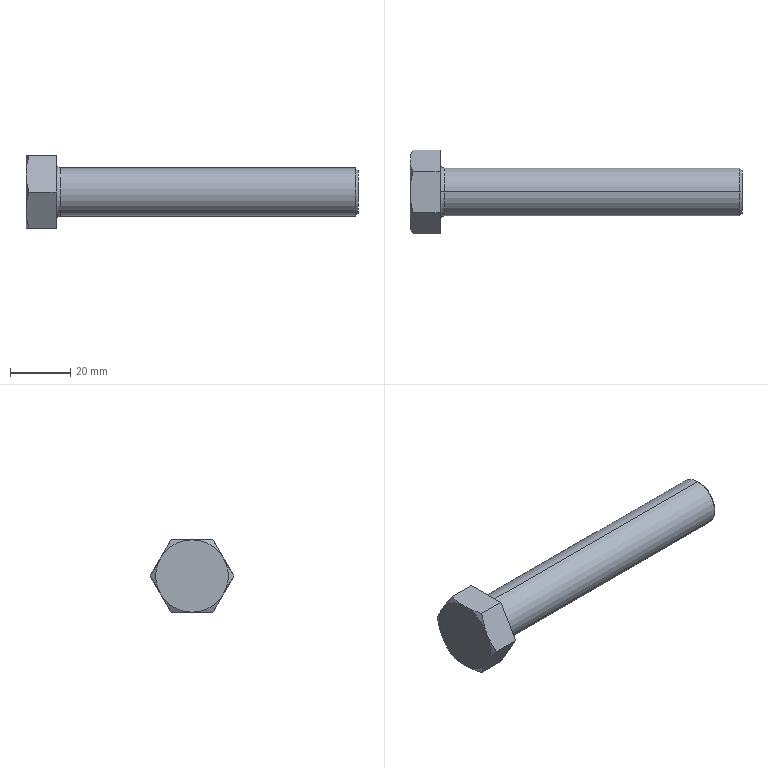Part | SolidWorks | features Chamfer 2, RevCut 2, Revolution 2, Extrusion 1, ICE 1 | 1 solid | 21 faces | box 110 x 27.713 x 24 mm | volume 25081 mm3 | plane 9 | cone 8 | cylinder 2 | torus 2 | commonest cylinder face diameters 16 x2
STEP:
#1=CARTESIAN_POINT('',(110.,0.,-7.111));
#2=VERTEX_POINT('',#1);
#3=CARTESIAN_POINT('',(110.,0.,7.111));
#4=VERTEX_POINT('',#3);
#5=CARTESIAN_POINT('',(110.,0.,0.));
#6=DIRECTION('',(1.,0.,0.));
#7=DIRECTION('',(0.,0.,1.));
#8=AXIS2_PLACEMENT_3D('',#5,#6,#7);
#9=CIRCLE('',#8,7.111);
#10=EDGE_CURVE('',#2,#4,#9,.T.);
#11=ORIENTED_EDGE('',*,*,#10,.F.);
#12=CARTESIAN_POINT('',(109.111,0.,-8.));
#13=VERTEX_POINT('',#12);
#14=CARTESIAN_POINT('',(109.111,0.,-8.));
#15=DIRECTION('',(-0.7071,0.,-0.7071));
#16=VECTOR('',#15,1000.);
#17=LINE('',#14,#16);
#18=EDGE_CURVE('',#2,#13,#17,.T.);
#19=ORIENTED_EDGE('',*,*,#18,.T.);
#20=CARTESIAN_POINT('',(109.111,0.,8.));
#21=VERTEX_POINT('',#20);
#22=CARTESIAN_POINT('',(109.111,0.,0.));
#23=DIRECTION('',(-1.,0.,0.));
#24=DIRECTION('',(0.,0.,1.));
#25=AXIS2_PLACEMENT_3D('',#22,#23,#24);
#26=CIRCLE('',#25,8.);
#27=EDGE_CURVE('',#21,#13,#26,.T.);
#28=ORIENTED_EDGE('',*,*,#27,.F.);
#29=CARTESIAN_POINT('',(109.111,0.,8.));
#30=DIRECTION('',(-0.7071,0.,0.7071));
#31=VECTOR('',#30,1000.);
#32=LINE('',#29,#31);
#33=EDGE_CURVE('',#4,#21,#32,.T.);
#34=ORIENTED_EDGE('',*,*,#33,.F.);
#35=EDGE_LOOP('',(#11,#19,#28,#34));
#36=FACE_OUTER_BOUND('',#35,.T.);
#37=CARTESIAN_POINT('',(109.111,0.,0.));
#38=DIRECTION('',(-1.,0.,0.));
#39=DIRECTION('',(0.,0.,1.));
#40=AXIS2_PLACEMENT_3D('',#37,#38,#39);
#41=CONICAL_SURFACE('',#40,8.,0.7854);
#42=ADVANCED_FACE('',(#36),#41,.T.);
#43=ORIENTED_EDGE('',*,*,#27,.T.);
#44=CARTESIAN_POINT('',(11.35,0.,-8.));
#45=VERTEX_POINT('',#44);
#46=CARTESIAN_POINT('',(10.,0.,-8.));
#47=DIRECTION('',(-1.,0.,0.));
#48=VECTOR('',#47,1000.);
#49=LINE('',#46,#48);
#50=EDGE_CURVE('',#13,#45,#49,.T.);
#51=ORIENTED_EDGE('',*,*,#50,.T.);
#52=CARTESIAN_POINT('',(11.35,0.,8.));
#53=VERTEX_POINT('',#52);
#54=CARTESIAN_POINT('',(11.35,0.,0.));
#55=DIRECTION('',(-1.,0.,0.));
#56=DIRECTION('',(0.,0.,1.));
#57=AXIS2_PLACEMENT_3D('',#54,#55,#56);
#58=CIRCLE('',#57,8.);
#59=EDGE_CURVE('',#53,#45,#58,.T.);
#60=ORIENTED_EDGE('',*,*,#59,.F.);
#61=CARTESIAN_POINT('',(10.,0.,8.));
#62=DIRECTION('',(-1.,0.,0.));
#63=VECTOR('',#62,1000.);
#64=LINE('',#61,#63);
#65=EDGE_CURVE('',#21,#53,#64,.T.);
#66=ORIENTED_EDGE('',*,*,#65,.F.);
#67=EDGE_LOOP('',(#43,#51,#60,#66));
#68=FACE_OUTER_BOUND('',#67,.T.);
#69=CARTESIAN_POINT('',(10.,0.,0.));
#70=DIRECTION('',(-1.,0.,0.));
#71=DIRECTION('',(0.,0.,1.));
#72=AXIS2_PLACEMENT_3D('',#69,#70,#71);
#73=CYLINDRICAL_SURFACE('',#72,8.);
#74=ADVANCED_FACE('',(#68),#73,.T.);
#75=CARTESIAN_POINT('',(10.,0.,-9.35));
#76=VERTEX_POINT('',#75);
#77=CARTESIAN_POINT('',(10.,0.,9.35));
#78=VERTEX_POINT('',#77);
#79=CARTESIAN_POINT('',(10.,0.,0.));
#80=DIRECTION('',(-1.,0.,0.));
#81=DIRECTION('',(0.,0.,1.));
#82=AXIS2_PLACEMENT_3D('',#79,#80,#81);
#83=CIRCLE('',#82,9.35);
#84=EDGE_CURVE('',#76,#78,#83,.T.);
#85=ORIENTED_EDGE('',*,*,#84,.F.);
#86=CARTESIAN_POINT('',(11.35,0.,-9.35));
#87=DIRECTION('',(0.,1.,0.));
#88=DIRECTION('',(0.,0.,1.));
#89=AXIS2_PLACEMENT_3D('',#86,#87,#88);
#90=CIRCLE('',#89,1.35);
#91=EDGE_CURVE('',#76,#45,#90,.T.);
#92=ORIENTED_EDGE('',*,*,#91,.T.);
#93=CARTESIAN_POINT('',(11.35,0.,0.));
#94=DIRECTION('',(-1.,0.,0.));
#95=DIRECTION('',(0.,0.,1.));
#96=AXIS2_PLACEMENT_3D('',#93,#94,#95);
#97=CIRCLE('',#96,8.);
#98=EDGE_CURVE('',#45,#53,#97,.T.);
#99=ORIENTED_EDGE('',*,*,#98,.T.);
#100=CARTESIAN_POINT('',(11.35,0.,9.35));
#101=DIRECTION('',(0.,-1.,0.));
#102=DIRECTION('',(0.,0.,-1.));
#103=AXIS2_PLACEMENT_3D('',#100,#101,#102);
#104=CIRCLE('',#103,1.35);
#105=EDGE_CURVE('',#78,#53,#104,.T.);
#106=ORIENTED_EDGE('',*,*,#105,.F.);
#107=EDGE_LOOP('',(#85,#92,#99,#106));
#108=FACE_OUTER_BOUND('',#107,.T.);
#109=CARTESIAN_POINT('',(11.35,0.,0.));
#110=DIRECTION('',(-1.,0.,0.));
#111=DIRECTION('',(0.,0.,1.));
#112=AXIS2_PLACEMENT_3D('',#109,#110,#111);
#113=TOROIDAL_SURFACE('',#112,9.35,1.35);
#114=ADVANCED_FACE('',(#108),#113,.F.);
#115=CARTESIAN_POINT('',(10.,-6.928,-12.));
#116=VERTEX_POINT('',#115);
#117=CARTESIAN_POINT('',(10.,6.928,-12.));
#118=VERTEX_POINT('',#117);
#119=CARTESIAN_POINT('',(10.,-6.928,-12.));
#120=DIRECTION('',(0.,1.,0.));
#121=VECTOR('',#120,1000.);
#122=LINE('',#119,#121);
#123=EDGE_CURVE('',#116,#118,#122,.T.);
#124=ORIENTED_EDGE('',*,*,#123,.T.);
#125=CARTESIAN_POINT('',(10.,13.856,0.));
#126=VERTEX_POINT('',#125);
#127=CARTESIAN_POINT('',(10.,6.928,-12.));
#128=DIRECTION('',(0.,0.5,0.866));
#129=VECTOR('',#128,1000.);
#130=LINE('',#127,#129);
#131=EDGE_CURVE('',#118,#126,#130,.T.);
#132=ORIENTED_EDGE('',*,*,#131,.T.);
#133=CARTESIAN_POINT('',(10.,6.928,12.));
#134=VERTEX_POINT('',#133);
#135=CARTESIAN_POINT('',(10.,13.856,0.));
#136=DIRECTION('',(0.,-0.5,0.866));
#137=VECTOR('',#136,1000.);
#138=LINE('',#135,#137);
#139=EDGE_CURVE('',#126,#134,#138,.T.);
#140=ORIENTED_EDGE('',*,*,#139,.T.);
#141=CARTESIAN_POINT('',(10.,-6.928,12.));
#142=VERTEX_POINT('',#141);
#143=CARTESIAN_POINT('',(10.,6.928,12.));
#144=DIRECTION('',(0.,-1.,0.));
#145=VECTOR('',#144,1000.);
#146=LINE('',#143,#145);
#147=EDGE_CURVE('',#134,#142,#146,.T.);
#148=ORIENTED_EDGE('',*,*,#147,.T.);
#149=CARTESIAN_POINT('',(10.,-13.856,0.));
#150=VERTEX_POINT('',#149);
#151=CARTESIAN_POINT('',(10.,-6.928,12.));
#152=DIRECTION('',(0.,-0.5,-0.866));
#153=VECTOR('',#152,1000.);
#154=LINE('',#151,#153);
#155=EDGE_CURVE('',#142,#150,#154,.T.);
#156=ORIENTED_EDGE('',*,*,#155,.T.);
#157=CARTESIAN_POINT('',(10.,-13.856,0.));
#158=DIRECTION('',(0.,0.5,-0.866));
#159=VECTOR('',#158,1000.);
#160=LINE('',#157,#159);
#161=EDGE_CURVE('',#150,#116,#160,.T.);
#162=ORIENTED_EDGE('',*,*,#161,.T.);
#163=EDGE_LOOP('',(#124,#132,#140,#148,#156,#162));
#164=FACE_OUTER_BOUND('',#163,.T.);
#165=CARTESIAN_POINT('',(10.,0.,0.));
#166=DIRECTION('',(-1.,0.,0.));
#167=DIRECTION('',(0.,0.,1.));
#168=AXIS2_PLACEMENT_3D('',#165,#166,#167);
#169=CIRCLE('',#168,9.35);
#170=EDGE_CURVE('',#78,#76,#169,.T.);
#171=ORIENTED_EDGE('',*,*,#170,.T.);
#172=ORIENTED_EDGE('',*,*,#84,.T.);
#173=EDGE_LOOP('',(#171,#172));
#174=FACE_BOUND('',#173,.T.);
#175=CARTESIAN_POINT('',(10.,6.928,-12.));
#176=DIRECTION('',(1.,0.,0.));
#177=DIRECTION('',(0.,0.,-1.));
#178=AXIS2_PLACEMENT_3D('',#175,#176,#177);
#179=PLANE('',#178);
#180=ADVANCED_FACE('',(#164,#174),#179,.T.);
#181=CARTESIAN_POINT('',(1.072,6.928,-12.));
#182=VERTEX_POINT('',#181);
#183=CARTESIAN_POINT('',(0.,0.,-12.));
#184=VERTEX_POINT('',#183);
#185=CARTESIAN_POINT('',(1.072,6.928,-12.));
#186=CARTESIAN_POINT('',(0.7484,5.808,-12.));
#187=CARTESIAN_POINT('',(0.4791,4.673,-12.));
#188=CARTESIAN_POINT('',(0.1974,2.937,-12.));
#189=CARTESIAN_POINT('',(0.1238,2.353,-12.));
#190=CARTESIAN_POINT('',(0.0249,1.173,-12.));
#191=CARTESIAN_POINT('',(0.,0.5858,-12.));
#192=CARTESIAN_POINT('',(0.,0.,-12.));
#193=B_SPLINE_CURVE_WITH_KNOTS('',3,(#185,#186,#187,#188,#189,#190,#191,#192),.UNSPECIFIED.,.F.,.F.,(4,2,2,4),(0.005049,0.008547,0.0103,0.01204),.UNSPECIFIED.);
#194=EDGE_CURVE('',#182,#184,#193,.T.);
#195=ORIENTED_EDGE('',*,*,#194,.F.);
#196=CARTESIAN_POINT('',(10.,6.928,-12.));
#197=DIRECTION('',(-1.,0.,0.));
#198=VECTOR('',#197,1000.);
#199=LINE('',#196,#198);
#200=EDGE_CURVE('',#118,#182,#199,.T.);
#201=ORIENTED_EDGE('',*,*,#200,.F.);
#202=ORIENTED_EDGE('',*,*,#123,.F.);
#203=CARTESIAN_POINT('',(1.072,-6.928,-12.));
#204=VERTEX_POINT('',#203);
#205=CARTESIAN_POINT('',(10.,-6.928,-12.));
#206=DIRECTION('',(-1.,0.,0.));
#207=VECTOR('',#206,1000.);
#208=LINE('',#205,#207);
#209=EDGE_CURVE('',#116,#204,#208,.T.);
#210=ORIENTED_EDGE('',*,*,#209,.T.);
#211=CARTESIAN_POINT('',(0.,0.,-12.));
#212=CARTESIAN_POINT('',(0.,-1.171,-12.));
#213=CARTESIAN_POINT('',(0.1006,-2.334,-12.));
#214=CARTESIAN_POINT('',(0.4737,-4.647,-12.));
#215=CARTESIAN_POINT('',(0.7465,-5.801,-12.));
#216=CARTESIAN_POINT('',(1.072,-6.928,-12.));
#217=B_SPLINE_CURVE_WITH_KNOTS('',3,(#211,#212,#213,#214,#215,#216),.UNSPECIFIED.,.F.,.F.,(4,2,4),(0.01204,0.01554,0.01904),.UNSPECIFIED.);
#218=EDGE_CURVE('',#184,#204,#217,.T.);
#219=ORIENTED_EDGE('',*,*,#218,.F.);
#220=EDGE_LOOP('',(#195,#201,#202,#210,#219));
#221=FACE_OUTER_BOUND('',#220,.T.);
#222=CARTESIAN_POINT('',(10.,-6.928,-12.));
#223=DIRECTION('',(0.,0.,1.));
#224=DIRECTION('',(0.,-1.,0.));
#225=AXIS2_PLACEMENT_3D('',#222,#223,#224);
#226=PLANE('',#225);
#227=ADVANCED_FACE('',(#221),#226,.F.);
#228=CARTESIAN_POINT('',(1.072,13.856,0.));
#229=VERTEX_POINT('',#228);
#230=CARTESIAN_POINT('',(0.,10.392,-6.));
#231=VERTEX_POINT('',#230);
#232=CARTESIAN_POINT('',(1.072,13.856,0.));
#233=CARTESIAN_POINT('',(0.7446,13.29,-0.9815));
#234=CARTESIAN_POINT('',(0.4751,12.719,-1.97));
#235=CARTESIAN_POINT('',(0.1021,11.565,-3.968));
#236=CARTESIAN_POINT('',(0.,10.982,-4.978));
#237=CARTESIAN_POINT('',(0.,10.392,-6.));
#238=B_SPLINE_CURVE_WITH_KNOTS('',3,(#232,#233,#234,#235,#236,#237),.UNSPECIFIED.,.F.,.F.,(4,2,4),(0.000000238,0.003505,0.00701),.UNSPECIFIED.);
#239=EDGE_CURVE('',#229,#231,#238,.T.);
#240=ORIENTED_EDGE('',*,*,#239,.F.);
#241=CARTESIAN_POINT('',(10.,13.856,0.));
#242=DIRECTION('',(-1.,0.,0.));
#243=VECTOR('',#242,1000.);
#244=LINE('',#241,#243);
#245=EDGE_CURVE('',#126,#229,#244,.T.);
#246=ORIENTED_EDGE('',*,*,#245,.F.);
#247=ORIENTED_EDGE('',*,*,#131,.F.);
#248=ORIENTED_EDGE('',*,*,#200,.T.);
#249=CARTESIAN_POINT('',(0.,10.392,-6.));
#250=CARTESIAN_POINT('',(0.,10.098,-6.509));
#251=CARTESIAN_POINT('',(0.02533,9.803,-7.021));
#252=CARTESIAN_POINT('',(0.1234,9.219,-8.033));
#253=CARTESIAN_POINT('',(0.196,8.929,-8.535));
#254=CARTESIAN_POINT('',(0.476,8.063,-10.034));
#255=CARTESIAN_POINT('',(0.7454,7.493,-11.021));
#256=CARTESIAN_POINT('',(1.072,6.928,-12.));
#257=B_SPLINE_CURVE_WITH_KNOTS('',3,(#249,#250,#251,#252,#253,#254,#255,#256),.UNSPECIFIED.,.F.,.F.,(4,2,2,4),(0.00701,0.008756,0.0105,0.01399),.UNSPECIFIED.);
#258=EDGE_CURVE('',#231,#182,#257,.T.);
#259=ORIENTED_EDGE('',*,*,#258,.F.);
#260=EDGE_LOOP('',(#240,#246,#247,#248,#259));
#261=FACE_OUTER_BOUND('',#260,.T.);
#262=CARTESIAN_POINT('',(10.,6.928,-12.));
#263=DIRECTION('',(0.,-0.866,0.5));
#264=DIRECTION('',(0.,-0.5,-0.866));
#265=AXIS2_PLACEMENT_3D('',#262,#263,#264);
#266=PLANE('',#265);
#267=ADVANCED_FACE('',(#261),#266,.F.);
#268=CARTESIAN_POINT('',(1.072,6.928,12.));
#269=VERTEX_POINT('',#268);
#270=CARTESIAN_POINT('',(0.,10.392,6.));
#271=VERTEX_POINT('',#270);
#272=CARTESIAN_POINT('',(1.072,6.928,12.));
#273=CARTESIAN_POINT('',(0.7446,7.495,11.018));
#274=CARTESIAN_POINT('',(0.4751,8.066,10.03));
#275=CARTESIAN_POINT('',(0.1021,9.219,8.032));
#276=CARTESIAN_POINT('',(0.,9.802,7.022));
#277=CARTESIAN_POINT('',(0.,10.392,6.));
#278=B_SPLINE_CURVE_WITH_KNOTS('',3,(#272,#273,#274,#275,#276,#277),.UNSPECIFIED.,.F.,.F.,(4,2,4),(0.000000238,0.003505,0.00701),.UNSPECIFIED.);
#279=EDGE_CURVE('',#269,#271,#278,.T.);
#280=ORIENTED_EDGE('',*,*,#279,.F.);
#281=CARTESIAN_POINT('',(10.,6.928,12.));
#282=DIRECTION('',(-1.,0.,0.));
#283=VECTOR('',#282,1000.);
#284=LINE('',#281,#283);
#285=EDGE_CURVE('',#134,#269,#284,.T.);
#286=ORIENTED_EDGE('',*,*,#285,.F.);
#287=ORIENTED_EDGE('',*,*,#139,.F.);
#288=ORIENTED_EDGE('',*,*,#245,.T.);
#289=CARTESIAN_POINT('',(0.,10.392,6.));
#290=CARTESIAN_POINT('',(0.,10.686,5.491));
#291=CARTESIAN_POINT('',(0.02533,10.982,4.979));
#292=CARTESIAN_POINT('',(0.1234,11.566,3.967));
#293=CARTESIAN_POINT('',(0.196,11.856,3.465));
#294=CARTESIAN_POINT('',(0.476,12.721,1.966));
#295=CARTESIAN_POINT('',(0.7454,13.291,0.9791));
#296=CARTESIAN_POINT('',(1.072,13.856,0.));
#297=B_SPLINE_CURVE_WITH_KNOTS('',3,(#289,#290,#291,#292,#293,#294,#295,#296),.UNSPECIFIED.,.F.,.F.,(4,2,2,4),(0.00701,0.008756,0.0105,0.01399),.UNSPECIFIED.);
#298=EDGE_CURVE('',#271,#229,#297,.T.);
#299=ORIENTED_EDGE('',*,*,#298,.F.);
#300=EDGE_LOOP('',(#280,#286,#287,#288,#299));
#301=FACE_OUTER_BOUND('',#300,.T.);
#302=CARTESIAN_POINT('',(10.,13.856,0.));
#303=DIRECTION('',(0.,-0.866,-0.5));
#304=DIRECTION('',(0.,0.5,-0.866));
#305=AXIS2_PLACEMENT_3D('',#302,#303,#304);
#306=PLANE('',#305);
#307=ADVANCED_FACE('',(#301),#306,.F.);
#308=CARTESIAN_POINT('',(1.072,-6.928,12.));
#309=VERTEX_POINT('',#308);
#310=CARTESIAN_POINT('',(0.,0.,12.));
#311=VERTEX_POINT('',#310);
#312=CARTESIAN_POINT('',(1.072,-6.928,12.));
#313=CARTESIAN_POINT('',(0.7465,-5.801,12.));
#314=CARTESIAN_POINT('',(0.4737,-4.647,12.));
#315=CARTESIAN_POINT('',(0.1006,-2.334,12.));
#316=CARTESIAN_POINT('',(0.,-1.171,12.));
#317=CARTESIAN_POINT('',(0.,0.,12.));
#318=B_SPLINE_CURVE_WITH_KNOTS('',3,(#312,#313,#314,#315,#316,#317),.UNSPECIFIED.,.F.,.F.,(4,2,4),(0.01239,0.01589,0.0194),.UNSPECIFIED.);
#319=EDGE_CURVE('',#309,#311,#318,.T.);
#320=ORIENTED_EDGE('',*,*,#319,.F.);
#321=CARTESIAN_POINT('',(10.,-6.928,12.));
#322=DIRECTION('',(-1.,0.,0.));
#323=VECTOR('',#322,1000.);
#324=LINE('',#321,#323);
#325=EDGE_CURVE('',#142,#309,#324,.T.);
#326=ORIENTED_EDGE('',*,*,#325,.F.);
#327=ORIENTED_EDGE('',*,*,#147,.F.);
#328=ORIENTED_EDGE('',*,*,#285,.T.);
#329=CARTESIAN_POINT('',(0.,0.,12.));
#330=CARTESIAN_POINT('',(0.,0.5858,12.));
#331=CARTESIAN_POINT('',(0.0249,1.173,12.));
#332=CARTESIAN_POINT('',(0.1238,2.353,12.));
#333=CARTESIAN_POINT('',(0.1974,2.937,12.));
#334=CARTESIAN_POINT('',(0.4791,4.673,12.));
#335=CARTESIAN_POINT('',(0.7484,5.808,12.));
#336=CARTESIAN_POINT('',(1.072,6.928,12.));
#337=B_SPLINE_CURVE_WITH_KNOTS('',3,(#329,#330,#331,#332,#333,#334,#335,#336),.UNSPECIFIED.,.F.,.F.,(4,2,2,4),(0.0194,0.02115,0.0229,0.02641),.UNSPECIFIED.);
#338=EDGE_CURVE('',#311,#269,#337,.T.);
#339=ORIENTED_EDGE('',*,*,#338,.F.);
#340=EDGE_LOOP('',(#320,#326,#327,#328,#339));
#341=FACE_OUTER_BOUND('',#340,.T.);
#342=CARTESIAN_POINT('',(10.,6.928,12.));
#343=DIRECTION('',(0.,0.,-1.));
#344=DIRECTION('',(0.,1.,0.));
#345=AXIS2_PLACEMENT_3D('',#342,#343,#344);
#346=PLANE('',#345);
#347=ADVANCED_FACE('',(#341),#346,.F.);
#348=CARTESIAN_POINT('',(1.072,-13.856,0.));
#349=VERTEX_POINT('',#348);
#350=CARTESIAN_POINT('',(0.,-10.392,6.));
#351=VERTEX_POINT('',#350);
#352=CARTESIAN_POINT('',(1.072,-13.856,0.));
#353=CARTESIAN_POINT('',(0.7446,-13.29,0.9815));
#354=CARTESIAN_POINT('',(0.4751,-12.719,1.97));
#355=CARTESIAN_POINT('',(0.1021,-11.565,3.968));
#356=CARTESIAN_POINT('',(0.,-10.982,4.978));
#357=CARTESIAN_POINT('',(0.,-10.392,6.));
#358=B_SPLINE_CURVE_WITH_KNOTS('',3,(#352,#353,#354,#355,#356,#357),.UNSPECIFIED.,.F.,.F.,(4,2,4),(0.000000238,0.003505,0.00701),.UNSPECIFIED.);
#359=EDGE_CURVE('',#349,#351,#358,.T.);
#360=ORIENTED_EDGE('',*,*,#359,.F.);
#361=CARTESIAN_POINT('',(10.,-13.856,0.));
#362=DIRECTION('',(-1.,0.,0.));
#363=VECTOR('',#362,1000.);
#364=LINE('',#361,#363);
#365=EDGE_CURVE('',#150,#349,#364,.T.);
#366=ORIENTED_EDGE('',*,*,#365,.F.);
#367=ORIENTED_EDGE('',*,*,#155,.F.);
#368=ORIENTED_EDGE('',*,*,#325,.T.);
#369=CARTESIAN_POINT('',(0.,-10.392,6.));
#370=CARTESIAN_POINT('',(0.,-10.098,6.509));
#371=CARTESIAN_POINT('',(0.02533,-9.803,7.021));
#372=CARTESIAN_POINT('',(0.1234,-9.219,8.033));
#373=CARTESIAN_POINT('',(0.196,-8.929,8.535));
#374=CARTESIAN_POINT('',(0.476,-8.063,10.034));
#375=CARTESIAN_POINT('',(0.7454,-7.493,11.021));
#376=CARTESIAN_POINT('',(1.072,-6.928,12.));
#377=B_SPLINE_CURVE_WITH_KNOTS('',3,(#369,#370,#371,#372,#373,#374,#375,#376),.UNSPECIFIED.,.F.,.F.,(4,2,2,4),(0.00701,0.008756,0.0105,0.01399),.UNSPECIFIED.);
#378=EDGE_CURVE('',#351,#309,#377,.T.);
#379=ORIENTED_EDGE('',*,*,#378,.F.);
#380=EDGE_LOOP('',(#360,#366,#367,#368,#379));
#381=FACE_OUTER_BOUND('',#380,.T.);
#382=CARTESIAN_POINT('',(10.,-6.928,12.));
#383=DIRECTION('',(0.,0.866,-0.5));
#384=DIRECTION('',(0.,0.5,0.866));
#385=AXIS2_PLACEMENT_3D('',#382,#383,#384);
#386=PLANE('',#385);
#387=ADVANCED_FACE('',(#381),#386,.F.);
#388=CARTESIAN_POINT('',(0.,-10.392,-6.));
#389=VERTEX_POINT('',#388);
#390=CARTESIAN_POINT('',(1.072,-6.928,-12.));
#391=CARTESIAN_POINT('',(0.7446,-7.495,-11.018));
#392=CARTESIAN_POINT('',(0.4751,-8.066,-10.03));
#393=CARTESIAN_POINT('',(0.1021,-9.219,-8.032));
#394=CARTESIAN_POINT('',(0.,-9.802,-7.022));
#395=CARTESIAN_POINT('',(0.,-10.392,-6.));
#396=B_SPLINE_CURVE_WITH_KNOTS('',3,(#390,#391,#392,#393,#394,#395),.UNSPECIFIED.,.F.,.F.,(4,2,4),(0.000000238,0.003505,0.00701),.UNSPECIFIED.);
#397=EDGE_CURVE('',#204,#389,#396,.T.);
#398=ORIENTED_EDGE('',*,*,#397,.F.);
#399=ORIENTED_EDGE('',*,*,#209,.F.);
#400=ORIENTED_EDGE('',*,*,#161,.F.);
#401=ORIENTED_EDGE('',*,*,#365,.T.);
#402=CARTESIAN_POINT('',(0.,-10.392,-6.));
#403=CARTESIAN_POINT('',(0.,-10.686,-5.491));
#404=CARTESIAN_POINT('',(0.02533,-10.982,-4.979));
#405=CARTESIAN_POINT('',(0.1234,-11.566,-3.967));
#406=CARTESIAN_POINT('',(0.196,-11.856,-3.465));
#407=CARTESIAN_POINT('',(0.476,-12.721,-1.966));
#408=CARTESIAN_POINT('',(0.7454,-13.291,-0.9791));
#409=CARTESIAN_POINT('',(1.072,-13.856,0.));
#410=B_SPLINE_CURVE_WITH_KNOTS('',3,(#402,#403,#404,#405,#406,#407,#408,#409),.UNSPECIFIED.,.F.,.F.,(4,2,2,4),(0.00701,0.008756,0.0105,0.01399),.UNSPECIFIED.);
#411=EDGE_CURVE('',#389,#349,#410,.T.);
#412=ORIENTED_EDGE('',*,*,#411,.F.);
#413=EDGE_LOOP('',(#398,#399,#400,#401,#412));
#414=FACE_OUTER_BOUND('',#413,.T.);
#415=CARTESIAN_POINT('',(10.,-13.856,0.));
#416=DIRECTION('',(0.,0.866,0.5));
#417=DIRECTION('',(0.,-0.5,0.866));
#418=AXIS2_PLACEMENT_3D('',#415,#416,#417);
#419=PLANE('',#418);
#420=ADVANCED_FACE('',(#414),#419,.F.);
#421=ORIENTED_EDGE('',*,*,#218,.T.);
#422=ORIENTED_EDGE('',*,*,#397,.T.);
#423=CARTESIAN_POINT('',(0.,0.,0.));
#424=DIRECTION('',(1.,0.,0.));
#425=DIRECTION('',(0.,0.,-1.));
#426=AXIS2_PLACEMENT_3D('',#423,#424,#425);
#427=CIRCLE('',#426,12.);
#428=EDGE_CURVE('',#389,#184,#427,.T.);
#429=ORIENTED_EDGE('',*,*,#428,.T.);
#430=EDGE_LOOP('',(#421,#422,#429));
#431=FACE_OUTER_BOUND('',#430,.T.);
#432=CARTESIAN_POINT('',(0.,0.,0.));
#433=DIRECTION('',(1.,0.,0.));
#434=DIRECTION('',(0.,0.,1.));
#435=AXIS2_PLACEMENT_3D('',#432,#433,#434);
#436=CONICAL_SURFACE('',#435,12.,1.047);
#437=ADVANCED_FACE('',(#431),#436,.T.);
#438=ORIENTED_EDGE('',*,*,#359,.T.);
#439=CARTESIAN_POINT('',(0.,0.,0.));
#440=DIRECTION('',(1.,0.,0.));
#441=DIRECTION('',(0.,0.,-1.));
#442=AXIS2_PLACEMENT_3D('',#439,#440,#441);
#443=CIRCLE('',#442,12.);
#444=EDGE_CURVE('',#351,#389,#443,.T.);
#445=ORIENTED_EDGE('',*,*,#444,.T.);
#446=ORIENTED_EDGE('',*,*,#411,.T.);
#447=EDGE_LOOP('',(#438,#445,#446));
#448=FACE_OUTER_BOUND('',#447,.T.);
#449=CARTESIAN_POINT('',(0.,0.,0.));
#450=DIRECTION('',(1.,0.,0.));
#451=DIRECTION('',(0.,0.,1.));
#452=AXIS2_PLACEMENT_3D('',#449,#450,#451);
#453=CONICAL_SURFACE('',#452,12.,1.047);
#454=ADVANCED_FACE('',(#448),#453,.T.);
#455=ORIENTED_EDGE('',*,*,#319,.T.);
#456=CARTESIAN_POINT('',(0.,0.,0.));
#457=DIRECTION('',(1.,0.,0.));
#458=DIRECTION('',(0.,0.,-1.));
#459=AXIS2_PLACEMENT_3D('',#456,#457,#458);
#460=CIRCLE('',#459,12.);
#461=EDGE_CURVE('',#311,#351,#460,.T.);
#462=ORIENTED_EDGE('',*,*,#461,.T.);
#463=ORIENTED_EDGE('',*,*,#378,.T.);
#464=EDGE_LOOP('',(#455,#462,#463));
#465=FACE_OUTER_BOUND('',#464,.T.);
#466=CARTESIAN_POINT('',(0.,0.,0.));
#467=DIRECTION('',(1.,0.,0.));
#468=DIRECTION('',(0.,0.,1.));
#469=AXIS2_PLACEMENT_3D('',#466,#467,#468);
#470=CONICAL_SURFACE('',#469,12.,1.047);
#471=ADVANCED_FACE('',(#465),#470,.T.);
#472=ORIENTED_EDGE('',*,*,#279,.T.);
#473=CARTESIAN_POINT('',(0.,0.,0.));
#474=DIRECTION('',(-1.,0.,0.));
#475=DIRECTION('',(0.,0.,1.));
#476=AXIS2_PLACEMENT_3D('',#473,#474,#475);
#477=CIRCLE('',#476,12.);
#478=EDGE_CURVE('',#311,#271,#477,.T.);
#479=ORIENTED_EDGE('',*,*,#478,.F.);
#480=ORIENTED_EDGE('',*,*,#338,.T.);
#481=EDGE_LOOP('',(#472,#479,#480));
#482=FACE_OUTER_BOUND('',#481,.T.);
#483=CARTESIAN_POINT('',(0.,0.,0.));
#484=DIRECTION('',(1.,0.,0.));
#485=DIRECTION('',(0.,0.,1.));
#486=AXIS2_PLACEMENT_3D('',#483,#484,#485);
#487=CONICAL_SURFACE('',#486,12.,1.047);
#488=ADVANCED_FACE('',(#482),#487,.T.);
#489=ORIENTED_EDGE('',*,*,#298,.T.);
#490=ORIENTED_EDGE('',*,*,#239,.T.);
#491=CARTESIAN_POINT('',(0.,0.,0.));
#492=DIRECTION('',(1.,0.,0.));
#493=DIRECTION('',(0.,0.,-1.));
#494=AXIS2_PLACEMENT_3D('',#491,#492,#493);
#495=CIRCLE('',#494,12.);
#496=EDGE_CURVE('',#231,#271,#495,.T.);
#497=ORIENTED_EDGE('',*,*,#496,.T.);
#498=EDGE_LOOP('',(#489,#490,#497));
#499=FACE_OUTER_BOUND('',#498,.T.);
#500=CARTESIAN_POINT('',(0.,0.,0.));
#501=DIRECTION('',(1.,0.,0.));
#502=DIRECTION('',(0.,0.,1.));
#503=AXIS2_PLACEMENT_3D('',#500,#501,#502);
#504=CONICAL_SURFACE('',#503,12.,1.047);
#505=ADVANCED_FACE('',(#499),#504,.T.);
#506=ORIENTED_EDGE('',*,*,#258,.T.);
#507=ORIENTED_EDGE('',*,*,#194,.T.);
#508=CARTESIAN_POINT('',(0.,0.,0.));
#509=DIRECTION('',(1.,0.,0.));
#510=DIRECTION('',(0.,0.,-1.));
#511=AXIS2_PLACEMENT_3D('',#508,#509,#510);
#512=CIRCLE('',#511,12.);
#513=EDGE_CURVE('',#184,#231,#512,.T.);
#514=ORIENTED_EDGE('',*,*,#513,.T.);
#515=EDGE_LOOP('',(#506,#507,#514));
#516=FACE_OUTER_BOUND('',#515,.T.);
#517=CARTESIAN_POINT('',(0.,0.,0.));
#518=DIRECTION('',(1.,0.,0.));
#519=DIRECTION('',(0.,0.,1.));
#520=AXIS2_PLACEMENT_3D('',#517,#518,#519);
#521=CONICAL_SURFACE('',#520,12.,1.047);
#522=ADVANCED_FACE('',(#516),#521,.T.);
#523=ORIENTED_EDGE('',*,*,#513,.F.);
#524=ORIENTED_EDGE('',*,*,#428,.F.);
#525=ORIENTED_EDGE('',*,*,#444,.F.);
#526=ORIENTED_EDGE('',*,*,#461,.F.);
#527=ORIENTED_EDGE('',*,*,#478,.T.);
#528=ORIENTED_EDGE('',*,*,#496,.F.);
#529=EDGE_LOOP('',(#523,#524,#525,#526,#527,#528));
#530=FACE_OUTER_BOUND('',#529,.T.);
#531=CARTESIAN_POINT('',(0.,6.928,-12.));
#532=DIRECTION('',(1.,0.,0.));
#533=DIRECTION('',(0.,0.,-1.));
#534=AXIS2_PLACEMENT_3D('',#531,#532,#533);
#535=PLANE('',#534);
#536=ADVANCED_FACE('',(#530),#535,.F.);
#537=ORIENTED_EDGE('',*,*,#91,.F.);
#538=ORIENTED_EDGE('',*,*,#170,.F.);
#539=ORIENTED_EDGE('',*,*,#105,.T.);
#540=ORIENTED_EDGE('',*,*,#59,.T.);
#541=EDGE_LOOP('',(#537,#538,#539,#540));
#542=FACE_OUTER_BOUND('',#541,.T.);
#543=CARTESIAN_POINT('',(11.35,0.,0.));
#544=DIRECTION('',(-1.,0.,0.));
#545=DIRECTION('',(0.,0.,1.));
#546=AXIS2_PLACEMENT_3D('',#543,#544,#545);
#547=TOROIDAL_SURFACE('',#546,9.35,1.35);
#548=ADVANCED_FACE('',(#542),#547,.F.);
#549=CARTESIAN_POINT('',(110.,0.,0.));
#550=DIRECTION('',(1.,0.,0.));
#551=DIRECTION('',(0.,0.,1.));
#552=AXIS2_PLACEMENT_3D('',#549,#550,#551);
#553=CIRCLE('',#552,7.111);
#554=EDGE_CURVE('',#4,#2,#553,.T.);
#555=ORIENTED_EDGE('',*,*,#554,.T.);
#556=ORIENTED_EDGE('',*,*,#10,.T.);
#557=EDGE_LOOP('',(#555,#556));
#558=FACE_OUTER_BOUND('',#557,.T.);
#559=CARTESIAN_POINT('',(110.,8.,0.));
#560=DIRECTION('',(-1.,0.,0.));
#561=DIRECTION('',(0.,0.,1.));
#562=AXIS2_PLACEMENT_3D('',#559,#560,#561);
#563=PLANE('',#562);
#564=ADVANCED_FACE('',(#558),#563,.F.);
#565=ORIENTED_EDGE('',*,*,#50,.F.);
#566=CARTESIAN_POINT('',(109.111,0.,0.));
#567=DIRECTION('',(-1.,0.,0.));
#568=DIRECTION('',(0.,0.,1.));
#569=AXIS2_PLACEMENT_3D('',#566,#567,#568);
#570=CIRCLE('',#569,8.);
#571=EDGE_CURVE('',#13,#21,#570,.T.);
#572=ORIENTED_EDGE('',*,*,#571,.T.);
#573=ORIENTED_EDGE('',*,*,#65,.T.);
#574=ORIENTED_EDGE('',*,*,#98,.F.);
#575=EDGE_LOOP('',(#565,#572,#573,#574));
#576=FACE_OUTER_BOUND('',#575,.T.);
#577=CARTESIAN_POINT('',(10.,0.,0.));
#578=DIRECTION('',(-1.,0.,0.));
#579=DIRECTION('',(0.,0.,1.));
#580=AXIS2_PLACEMENT_3D('',#577,#578,#579);
#581=CYLINDRICAL_SURFACE('',#580,8.);
#582=ADVANCED_FACE('',(#576),#581,.T.);
#583=ORIENTED_EDGE('',*,*,#18,.F.);
#584=ORIENTED_EDGE('',*,*,#554,.F.);
#585=ORIENTED_EDGE('',*,*,#33,.T.);
#586=ORIENTED_EDGE('',*,*,#571,.F.);
#587=EDGE_LOOP('',(#583,#584,#585,#586));
#588=FACE_OUTER_BOUND('',#587,.T.);
#589=CARTESIAN_POINT('',(109.111,0.,0.));
#590=DIRECTION('',(-1.,0.,0.));
#591=DIRECTION('',(0.,0.,1.));
#592=AXIS2_PLACEMENT_3D('',#589,#590,#591);
#593=CONICAL_SURFACE('',#592,8.,0.7854);
#594=ADVANCED_FACE('',(#588),#593,.T.);
#595=CLOSED_SHELL('',(#42,#74,#114,#180,#227,#267,#307,#347,#387,#420,#437,#454,#471,#488,#505,#522,#536,#548,#564,#582,#594));
#596=MANIFOLD_SOLID_BREP('',#595);
#597=CARTESIAN_POINT('',(0.,0.,0.));
#598=DIRECTION('',(0.,0.,1.));
#599=DIRECTION('',(1.,0.,0.));
#600=AXIS2_PLACEMENT_3D('',#597,#598,#599);
#601=(LENGTH_UNIT()NAMED_UNIT(*)SI_UNIT(.MILLI.,.METRE.));
#602=UNCERTAINTY_MEASURE_WITH_UNIT(LENGTH_MEASURE(0.00001),#601,'','');
#603=(NAMED_UNIT(*)PLANE_ANGLE_UNIT()SI_UNIT($,.RADIAN.));
#604=(NAMED_UNIT(*)SI_UNIT($,.STERADIAN.)SOLID_ANGLE_UNIT());
#605=(GEOMETRIC_REPRESENTATION_CONTEXT(3)GLOBAL_UNCERTAINTY_ASSIGNED_CONTEXT((#602))GLOBAL_UNIT_ASSIGNED_CONTEXT((#601,#603,#604))REPRESENTATION_CONTEXT('',''));
#606=ADVANCED_BREP_SHAPE_REPRESENTATION('',(#596,#600),#605);